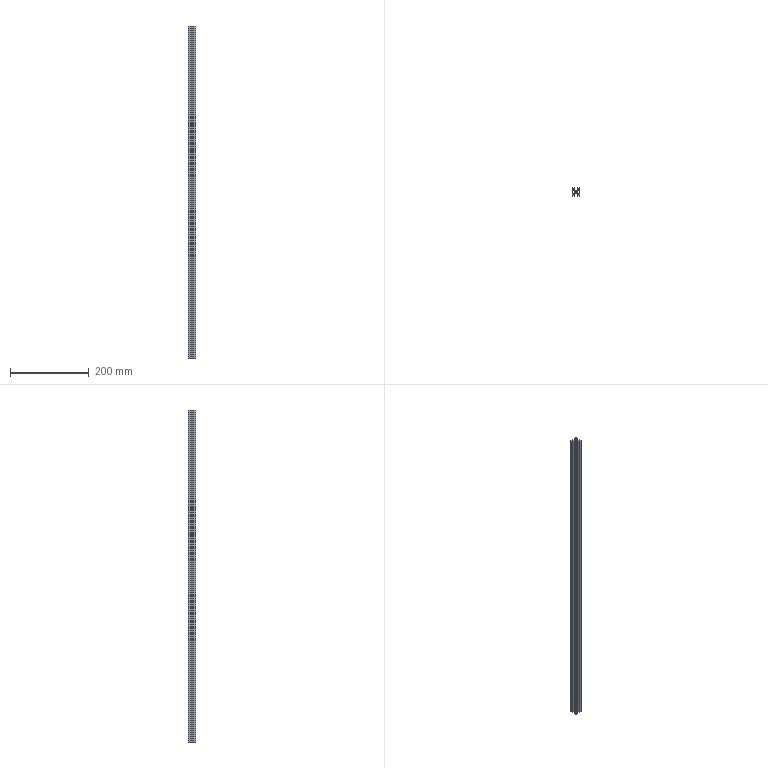Part | STEP file | AOB02-H2020_YHD010 | 1 solid | 80 faces | box 20 x 20 x 842 mm | volume 145364 mm3 | plane 74 | cylinder 6 | commonest cylinder face diameters 3 x4 5 x2